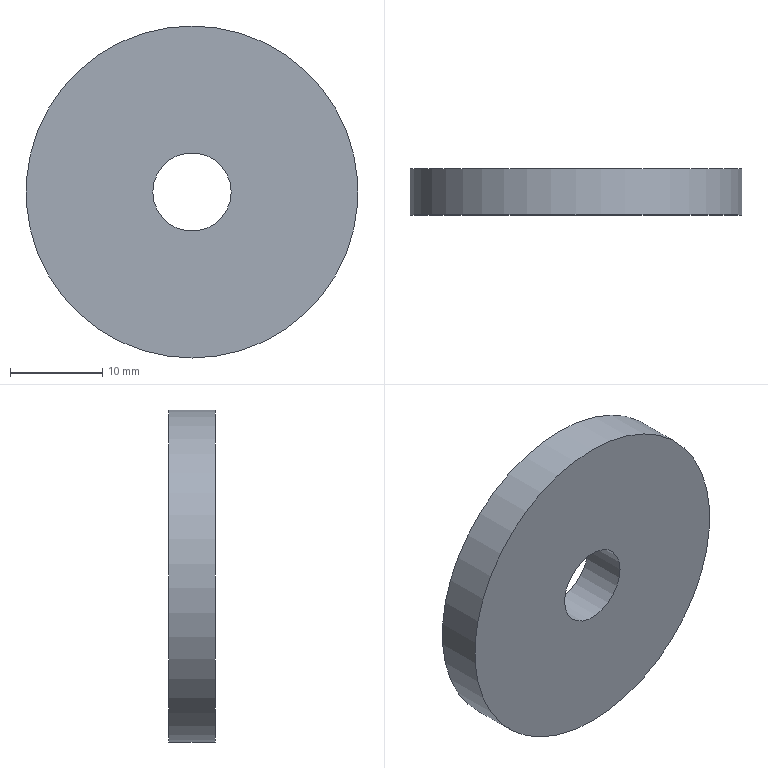Part | STEP file | 冲床-300配套压波_id458_x_t | 1 solid | 4 faces | box 36 x 5 x 36 mm | volume 4806 mm3 | cylinder 2 | plane 2 | commonest cylinder face diameters 8.5 x1 36 x1
STEP:
#1=CARTESIAN_POINT('',(1126.,-108.,-121.));
#2=VERTEX_POINT('',#1);
#3=CARTESIAN_POINT('',(1126.,-108.,-103.));
#4=DIRECTION('',(0.,-1.,0.));
#5=DIRECTION('',(0.,0.,-1.));
#6=AXIS2_PLACEMENT_3D('',#3,#4,#5);
#7=CIRCLE('',#6,18.);
#8=EDGE_CURVE('',#2,#2,#7,.T.);
#9=ORIENTED_EDGE('',*,*,#8,.T.);
#10=EDGE_LOOP('',(#9));
#11=FACE_BOUND('',#10,.T.);
#12=CARTESIAN_POINT('',(1126.,-113.,-121.));
#13=VERTEX_POINT('',#12);
#14=CARTESIAN_POINT('',(1126.,-113.,-103.));
#15=DIRECTION('',(0.,-1.,0.));
#16=DIRECTION('',(0.,0.,-1.));
#17=AXIS2_PLACEMENT_3D('',#14,#15,#16);
#18=CIRCLE('',#17,18.);
#19=EDGE_CURVE('',#13,#13,#18,.T.);
#20=ORIENTED_EDGE('',*,*,#19,.F.);
#21=EDGE_LOOP('',(#20));
#22=FACE_BOUND('',#21,.T.);
#23=CARTESIAN_POINT('',(1126.,-108.,-103.));
#24=DIRECTION('',(0.,-1.,0.));
#25=DIRECTION('',(-1.,0.,0.));
#26=AXIS2_PLACEMENT_3D('',#23,#24,#25);
#27=CYLINDRICAL_SURFACE('',#26,18.);
#28=ADVANCED_FACE('',(#11,#22),#27,.T.);
#29=CARTESIAN_POINT('',(1121.75,-108.,-103.));
#30=VERTEX_POINT('',#29);
#31=CARTESIAN_POINT('',(1126.,-108.,-103.));
#32=DIRECTION('',(0.,1.,0.));
#33=DIRECTION('',(-1.,0.,0.));
#34=AXIS2_PLACEMENT_3D('',#31,#32,#33);
#35=CIRCLE('',#34,4.25);
#36=EDGE_CURVE('',#30,#30,#35,.T.);
#37=ORIENTED_EDGE('',*,*,#36,.F.);
#38=EDGE_LOOP('',(#37));
#39=FACE_BOUND('',#38,.T.);
#40=ORIENTED_EDGE('',*,*,#8,.F.);
#41=EDGE_LOOP('',(#40));
#42=FACE_BOUND('',#41,.T.);
#43=CARTESIAN_POINT('',(1126.,-108.,-103.));
#44=DIRECTION('',(0.,-1.,0.));
#45=DIRECTION('',(-1.,0.,0.));
#46=AXIS2_PLACEMENT_3D('',#43,#44,#45);
#47=PLANE('',#46);
#48=ADVANCED_FACE('',(#39,#42),#47,.F.);
#49=CARTESIAN_POINT('',(1121.75,-113.,-103.));
#50=VERTEX_POINT('',#49);
#51=CARTESIAN_POINT('',(1126.,-113.,-103.));
#52=DIRECTION('',(0.,1.,0.));
#53=DIRECTION('',(-1.,0.,0.));
#54=AXIS2_PLACEMENT_3D('',#51,#52,#53);
#55=CIRCLE('',#54,4.25);
#56=EDGE_CURVE('',#50,#50,#55,.T.);
#57=ORIENTED_EDGE('',*,*,#56,.T.);
#58=EDGE_LOOP('',(#57));
#59=FACE_BOUND('',#58,.T.);
#60=ORIENTED_EDGE('',*,*,#19,.T.);
#61=EDGE_LOOP('',(#60));
#62=FACE_BOUND('',#61,.T.);
#63=CARTESIAN_POINT('',(1126.,-113.,-103.));
#64=DIRECTION('',(0.,-1.,0.));
#65=DIRECTION('',(-1.,0.,0.));
#66=AXIS2_PLACEMENT_3D('',#63,#64,#65);
#67=PLANE('',#66);
#68=ADVANCED_FACE('',(#59,#62),#67,.T.);
#69=ORIENTED_EDGE('',*,*,#56,.F.);
#70=EDGE_LOOP('',(#69));
#71=FACE_BOUND('',#70,.T.);
#72=ORIENTED_EDGE('',*,*,#36,.T.);
#73=EDGE_LOOP('',(#72));
#74=FACE_BOUND('',#73,.T.);
#75=CARTESIAN_POINT('',(1126.,-49.,-103.));
#76=DIRECTION('',(0.,-1.,0.));
#77=DIRECTION('',(-1.,0.,0.));
#78=AXIS2_PLACEMENT_3D('',#75,#76,#77);
#79=CYLINDRICAL_SURFACE('',#78,4.25);
#80=ADVANCED_FACE('',(#71,#74),#79,.F.);
#81=CLOSED_SHELL('',(#28,#48,#68,#80));
#82=MANIFOLD_SOLID_BREP('',#81);
#83=(LENGTH_UNIT()NAMED_UNIT(*)SI_UNIT(.MILLI.,.METRE.));
#84=UNCERTAINTY_MEASURE_WITH_UNIT(LENGTH_MEASURE(0.00002),#83,'','');
#85=(NAMED_UNIT(*)PLANE_ANGLE_UNIT()SI_UNIT($,.RADIAN.));
#86=PLANE_ANGLE_MEASURE_WITH_UNIT(PLANE_ANGLE_MEASURE(0.01745),#85);
#87=DIMENSIONAL_EXPONENTS(0.,0.,0.,0.,0.,0.,0.);
#88=(CONVERSION_BASED_UNIT('DEGREE',#86)NAMED_UNIT(#87)PLANE_ANGLE_UNIT());
#89=(NAMED_UNIT(*)SI_UNIT($,.STERADIAN.)SOLID_ANGLE_UNIT());
#90=(GEOMETRIC_REPRESENTATION_CONTEXT(3)GLOBAL_UNCERTAINTY_ASSIGNED_CONTEXT((#84))GLOBAL_UNIT_ASSIGNED_CONTEXT((#83,#88,#89))REPRESENTATION_CONTEXT('',''));
#91=ADVANCED_BREP_SHAPE_REPRESENTATION('',(#82),#90);